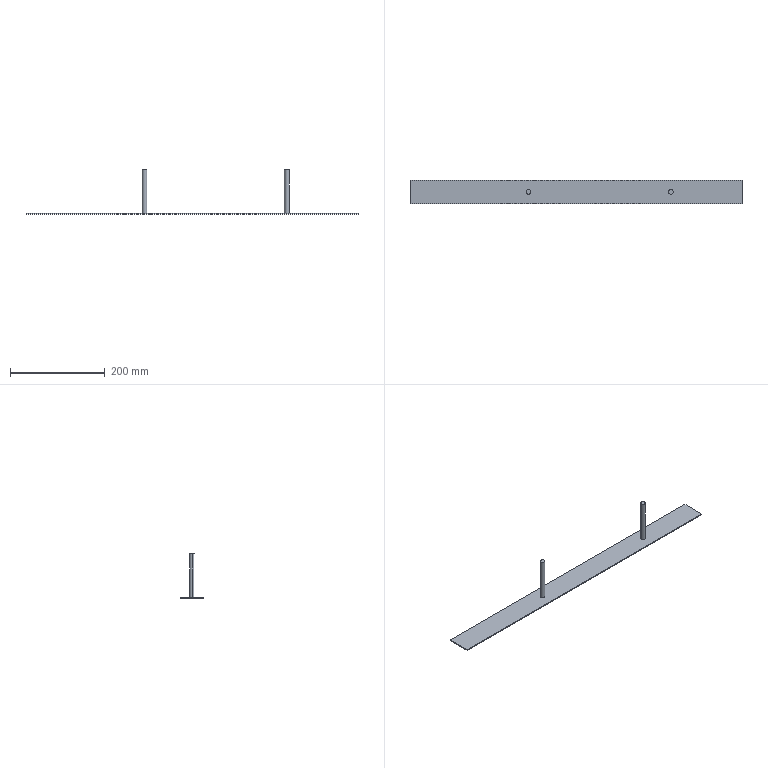Part | STEP file | 1 solid | 12 faces | box 700 x 50 x 93 mm | volume 84294 mm3 | plane 8 | cylinder 4 | commonest cylinder face diameters 10 x4
STEP:
#1=CARTESIAN_POINT('',(0.,0.,0.));
#2=DIRECTION('',(0.,0.,1.));
#3=DIRECTION('',(1.,0.,0.));
#4=AXIS2_PLACEMENT_3D('',#1,#2,#3);
#5=CARTESIAN_POINT('',(195.,0.,2.));
#6=VERTEX_POINT('',#5);
#7=CARTESIAN_POINT('',(205.,0.,2.));
#8=VERTEX_POINT('',#7);
#9=CARTESIAN_POINT('',(200.,0.,2.));
#10=DIRECTION('',(0.,0.,-1.));
#11=DIRECTION('',(1.,0.,0.));
#12=AXIS2_PLACEMENT_3D('',#9,#10,#11);
#13=CIRCLE('',#12,5.);
#14=CARTESIAN_POINT('',(200.,0.,93.));
#15=DIRECTION('',(0.,0.,1.));
#16=DIRECTION('',(1.,0.,0.));
#17=AXIS2_PLACEMENT_3D('',#14,#15,#16);
#18=CYLINDRICAL_SURFACE('',#17,5.);
#19=CARTESIAN_POINT('',(6.283,-91.));
#20=DIRECTION('',(-1.,0.));
#21=VECTOR('',#20,1.);
#22=LINE('',#19,#21);
#23=(GEOMETRIC_REPRESENTATION_CONTEXT(2)PARAMETRIC_REPRESENTATION_CONTEXT()REPRESENTATION_CONTEXT('',''));
#24=DEFINITIONAL_REPRESENTATION('',(#22),#23);
#25=PCURVE('',#18,#24);
#26=CARTESIAN_POINT('',(0.,0.,2.));
#27=DIRECTION('',(0.,0.,1.));
#28=DIRECTION('',(1.,0.,0.));
#29=AXIS2_PLACEMENT_3D('',#26,#27,#28);
#30=PLANE('',#29);
#31=CARTESIAN_POINT('',(205.,0.));
#32=CARTESIAN_POINT('',(205.,-8.66));
#33=CARTESIAN_POINT('',(197.5,-4.33));
#34=CARTESIAN_POINT('',(190.,0.));
#35=CARTESIAN_POINT('',(197.5,4.33));
#36=CARTESIAN_POINT('',(205.,8.66));
#37=CARTESIAN_POINT('',(205.,0.));
#38=(BOUNDED_CURVE()B_SPLINE_CURVE(2,(#31,#32,#33,#34,#35,#36,#37),.UNSPECIFIED.,.T.,.F.)B_SPLINE_CURVE_WITH_KNOTS((1,2,2,2,2,1),(-2.094,0.,2.094,4.189,6.283,8.378),.UNSPECIFIED.)CURVE()GEOMETRIC_REPRESENTATION_ITEM()RATIONAL_B_SPLINE_CURVE((1.,0.5,1.,0.5,1.,0.5,1.))REPRESENTATION_ITEM(''));
#39=(GEOMETRIC_REPRESENTATION_CONTEXT(2)PARAMETRIC_REPRESENTATION_CONTEXT()REPRESENTATION_CONTEXT('',''));
#40=DEFINITIONAL_REPRESENTATION('',(#38),#39);
#41=PCURVE('',#30,#40);
#42=SURFACE_CURVE('',#13,(#25,#41),.PCURVE_S1.);
#43=EDGE_CURVE('',#6,#8,#42,.T.);
#44=ORIENTED_EDGE('',*,*,#43,.F.);
#45=CARTESIAN_POINT('',(195.,0.,93.));
#46=VERTEX_POINT('',#45);
#47=CARTESIAN_POINT('',(195.,0.,93.));
#48=DIRECTION('',(0.,0.,1.));
#49=VECTOR('',#48,1.);
#50=LINE('',#47,#49);
#51=CARTESIAN_POINT('',(3.142,0.));
#52=DIRECTION('',(0.,1.));
#53=VECTOR('',#52,1.);
#54=LINE('',#51,#53);
#55=(GEOMETRIC_REPRESENTATION_CONTEXT(2)PARAMETRIC_REPRESENTATION_CONTEXT()REPRESENTATION_CONTEXT('',''));
#56=DEFINITIONAL_REPRESENTATION('',(#54),#55);
#57=PCURVE('',#18,#56);
#58=CARTESIAN_POINT('',(200.,0.,93.));
#59=DIRECTION('',(0.,0.,1.));
#60=DIRECTION('',(1.,0.,0.));
#61=AXIS2_PLACEMENT_3D('',#58,#59,#60);
#62=CYLINDRICAL_SURFACE('',#61,5.);
#63=CARTESIAN_POINT('',(3.142,0.));
#64=DIRECTION('',(0.,1.));
#65=VECTOR('',#64,1.);
#66=LINE('',#63,#65);
#67=(GEOMETRIC_REPRESENTATION_CONTEXT(2)PARAMETRIC_REPRESENTATION_CONTEXT()REPRESENTATION_CONTEXT('',''));
#68=DEFINITIONAL_REPRESENTATION('',(#66),#67);
#69=PCURVE('',#62,#68);
#70=SURFACE_CURVE('',#50,(#57,#69),.PCURVE_S1.);
#71=EDGE_CURVE('',#6,#46,#70,.T.);
#72=ORIENTED_EDGE('',*,*,#71,.T.);
#73=CARTESIAN_POINT('',(205.,0.,93.));
#74=VERTEX_POINT('',#73);
#75=CARTESIAN_POINT('',(200.,0.,93.));
#76=DIRECTION('',(0.,0.,-1.));
#77=DIRECTION('',(1.,0.,0.));
#78=AXIS2_PLACEMENT_3D('',#75,#76,#77);
#79=CIRCLE('',#78,5.);
#80=CARTESIAN_POINT('',(6.283,0.));
#81=DIRECTION('',(-1.,0.));
#82=VECTOR('',#81,1.);
#83=LINE('',#80,#82);
#84=(GEOMETRIC_REPRESENTATION_CONTEXT(2)PARAMETRIC_REPRESENTATION_CONTEXT()REPRESENTATION_CONTEXT('',''));
#85=DEFINITIONAL_REPRESENTATION('',(#83),#84);
#86=PCURVE('',#18,#85);
#87=CARTESIAN_POINT('',(200.,0.,93.));
#88=DIRECTION('',(0.,0.,1.));
#89=DIRECTION('',(1.,0.,0.));
#90=AXIS2_PLACEMENT_3D('',#87,#88,#89);
#91=PLANE('',#90);
#92=CARTESIAN_POINT('',(5.,0.));
#93=CARTESIAN_POINT('',(5.,-8.66));
#94=CARTESIAN_POINT('',(-2.5,-4.33));
#95=CARTESIAN_POINT('',(-10.,0.));
#96=CARTESIAN_POINT('',(-2.5,4.33));
#97=CARTESIAN_POINT('',(5.,8.66));
#98=CARTESIAN_POINT('',(5.,0.));
#99=(BOUNDED_CURVE()B_SPLINE_CURVE(2,(#92,#93,#94,#95,#96,#97,#98),.UNSPECIFIED.,.T.,.F.)B_SPLINE_CURVE_WITH_KNOTS((1,2,2,2,2,1),(-2.094,0.,2.094,4.189,6.283,8.378),.UNSPECIFIED.)CURVE()GEOMETRIC_REPRESENTATION_ITEM()RATIONAL_B_SPLINE_CURVE((1.,0.5,1.,0.5,1.,0.5,1.))REPRESENTATION_ITEM(''));
#100=(GEOMETRIC_REPRESENTATION_CONTEXT(2)PARAMETRIC_REPRESENTATION_CONTEXT()REPRESENTATION_CONTEXT('',''));
#101=DEFINITIONAL_REPRESENTATION('',(#99),#100);
#102=PCURVE('',#91,#101);
#103=SURFACE_CURVE('',#79,(#86,#102),.PCURVE_S1.);
#104=EDGE_CURVE('',#46,#74,#103,.T.);
#105=ORIENTED_EDGE('',*,*,#104,.T.);
#106=CARTESIAN_POINT('',(205.,0.,93.));
#107=DIRECTION('',(0.,0.,1.));
#108=VECTOR('',#107,1.);
#109=LINE('',#106,#108);
#110=CARTESIAN_POINT('',(0.,0.));
#111=DIRECTION('',(0.,1.));
#112=VECTOR('',#111,1.);
#113=LINE('',#110,#112);
#114=(GEOMETRIC_REPRESENTATION_CONTEXT(2)PARAMETRIC_REPRESENTATION_CONTEXT()REPRESENTATION_CONTEXT('',''));
#115=DEFINITIONAL_REPRESENTATION('',(#113),#114);
#116=PCURVE('',#18,#115);
#117=CARTESIAN_POINT('',(6.283,0.));
#118=DIRECTION('',(0.,1.));
#119=VECTOR('',#118,1.);
#120=LINE('',#117,#119);
#121=(GEOMETRIC_REPRESENTATION_CONTEXT(2)PARAMETRIC_REPRESENTATION_CONTEXT()REPRESENTATION_CONTEXT('',''));
#122=DEFINITIONAL_REPRESENTATION('',(#120),#121);
#123=PCURVE('',#62,#122);
#124=SURFACE_CURVE('',#109,(#116,#123),.PCURVE_S1.);
#125=EDGE_CURVE('',#8,#74,#124,.T.);
#126=ORIENTED_EDGE('',*,*,#125,.F.);
#127=EDGE_LOOP('',(#44,#72,#105,#126));
#128=FACE_BOUND('',#127,.T.);
#129=ADVANCED_FACE('',(#128),#18,.T.);
#130=CARTESIAN_POINT('',(-105.,0.,2.));
#131=VERTEX_POINT('',#130);
#132=CARTESIAN_POINT('',(-95.,0.,2.));
#133=VERTEX_POINT('',#132);
#134=CARTESIAN_POINT('',(-100.,0.,2.));
#135=DIRECTION('',(0.,0.,-1.));
#136=DIRECTION('',(1.,0.,0.));
#137=AXIS2_PLACEMENT_3D('',#134,#135,#136);
#138=CIRCLE('',#137,5.);
#139=CARTESIAN_POINT('',(-100.,0.,93.));
#140=DIRECTION('',(0.,0.,1.));
#141=DIRECTION('',(1.,0.,0.));
#142=AXIS2_PLACEMENT_3D('',#139,#140,#141);
#143=CYLINDRICAL_SURFACE('',#142,5.);
#144=CARTESIAN_POINT('',(6.283,-91.));
#145=DIRECTION('',(-1.,0.));
#146=VECTOR('',#145,1.);
#147=LINE('',#144,#146);
#148=(GEOMETRIC_REPRESENTATION_CONTEXT(2)PARAMETRIC_REPRESENTATION_CONTEXT()REPRESENTATION_CONTEXT('',''));
#149=DEFINITIONAL_REPRESENTATION('',(#147),#148);
#150=PCURVE('',#143,#149);
#151=CARTESIAN_POINT('',(-95.,0.));
#152=CARTESIAN_POINT('',(-95.,-8.66));
#153=CARTESIAN_POINT('',(-102.5,-4.33));
#154=CARTESIAN_POINT('',(-110.,0.));
#155=CARTESIAN_POINT('',(-102.5,4.33));
#156=CARTESIAN_POINT('',(-95.,8.66));
#157=CARTESIAN_POINT('',(-95.,0.));
#158=(BOUNDED_CURVE()B_SPLINE_CURVE(2,(#151,#152,#153,#154,#155,#156,#157),.UNSPECIFIED.,.T.,.F.)B_SPLINE_CURVE_WITH_KNOTS((1,2,2,2,2,1),(-2.094,0.,2.094,4.189,6.283,8.378),.UNSPECIFIED.)CURVE()GEOMETRIC_REPRESENTATION_ITEM()RATIONAL_B_SPLINE_CURVE((1.,0.5,1.,0.5,1.,0.5,1.))REPRESENTATION_ITEM(''));
#159=(GEOMETRIC_REPRESENTATION_CONTEXT(2)PARAMETRIC_REPRESENTATION_CONTEXT()REPRESENTATION_CONTEXT('',''));
#160=DEFINITIONAL_REPRESENTATION('',(#158),#159);
#161=PCURVE('',#30,#160);
#162=SURFACE_CURVE('',#138,(#150,#161),.PCURVE_S1.);
#163=EDGE_CURVE('',#131,#133,#162,.T.);
#164=ORIENTED_EDGE('',*,*,#163,.F.);
#165=CARTESIAN_POINT('',(-105.,0.,93.));
#166=VERTEX_POINT('',#165);
#167=CARTESIAN_POINT('',(-105.,0.,93.));
#168=DIRECTION('',(0.,0.,1.));
#169=VECTOR('',#168,1.);
#170=LINE('',#167,#169);
#171=CARTESIAN_POINT('',(3.142,0.));
#172=DIRECTION('',(0.,1.));
#173=VECTOR('',#172,1.);
#174=LINE('',#171,#173);
#175=(GEOMETRIC_REPRESENTATION_CONTEXT(2)PARAMETRIC_REPRESENTATION_CONTEXT()REPRESENTATION_CONTEXT('',''));
#176=DEFINITIONAL_REPRESENTATION('',(#174),#175);
#177=PCURVE('',#143,#176);
#178=CARTESIAN_POINT('',(-100.,0.,93.));
#179=DIRECTION('',(0.,0.,1.));
#180=DIRECTION('',(1.,0.,0.));
#181=AXIS2_PLACEMENT_3D('',#178,#179,#180);
#182=CYLINDRICAL_SURFACE('',#181,5.);
#183=CARTESIAN_POINT('',(3.142,0.));
#184=DIRECTION('',(0.,1.));
#185=VECTOR('',#184,1.);
#186=LINE('',#183,#185);
#187=(GEOMETRIC_REPRESENTATION_CONTEXT(2)PARAMETRIC_REPRESENTATION_CONTEXT()REPRESENTATION_CONTEXT('',''));
#188=DEFINITIONAL_REPRESENTATION('',(#186),#187);
#189=PCURVE('',#182,#188);
#190=SURFACE_CURVE('',#170,(#177,#189),.PCURVE_S1.);
#191=EDGE_CURVE('',#131,#166,#190,.T.);
#192=ORIENTED_EDGE('',*,*,#191,.T.);
#193=CARTESIAN_POINT('',(-95.,0.,93.));
#194=VERTEX_POINT('',#193);
#195=CARTESIAN_POINT('',(-100.,0.,93.));
#196=DIRECTION('',(0.,0.,-1.));
#197=DIRECTION('',(1.,0.,0.));
#198=AXIS2_PLACEMENT_3D('',#195,#196,#197);
#199=CIRCLE('',#198,5.);
#200=CARTESIAN_POINT('',(6.283,0.));
#201=DIRECTION('',(-1.,0.));
#202=VECTOR('',#201,1.);
#203=LINE('',#200,#202);
#204=(GEOMETRIC_REPRESENTATION_CONTEXT(2)PARAMETRIC_REPRESENTATION_CONTEXT()REPRESENTATION_CONTEXT('',''));
#205=DEFINITIONAL_REPRESENTATION('',(#203),#204);
#206=PCURVE('',#143,#205);
#207=CARTESIAN_POINT('',(-100.,0.,93.));
#208=DIRECTION('',(0.,0.,1.));
#209=DIRECTION('',(1.,0.,0.));
#210=AXIS2_PLACEMENT_3D('',#207,#208,#209);
#211=PLANE('',#210);
#212=CARTESIAN_POINT('',(5.,0.));
#213=CARTESIAN_POINT('',(5.,-8.66));
#214=CARTESIAN_POINT('',(-2.5,-4.33));
#215=CARTESIAN_POINT('',(-10.,0.));
#216=CARTESIAN_POINT('',(-2.5,4.33));
#217=CARTESIAN_POINT('',(5.,8.66));
#218=CARTESIAN_POINT('',(5.,0.));
#219=(BOUNDED_CURVE()B_SPLINE_CURVE(2,(#212,#213,#214,#215,#216,#217,#218),.UNSPECIFIED.,.T.,.F.)B_SPLINE_CURVE_WITH_KNOTS((1,2,2,2,2,1),(-2.094,0.,2.094,4.189,6.283,8.378),.UNSPECIFIED.)CURVE()GEOMETRIC_REPRESENTATION_ITEM()RATIONAL_B_SPLINE_CURVE((1.,0.5,1.,0.5,1.,0.5,1.))REPRESENTATION_ITEM(''));
#220=(GEOMETRIC_REPRESENTATION_CONTEXT(2)PARAMETRIC_REPRESENTATION_CONTEXT()REPRESENTATION_CONTEXT('',''));
#221=DEFINITIONAL_REPRESENTATION('',(#219),#220);
#222=PCURVE('',#211,#221);
#223=SURFACE_CURVE('',#199,(#206,#222),.PCURVE_S1.);
#224=EDGE_CURVE('',#166,#194,#223,.T.);
#225=ORIENTED_EDGE('',*,*,#224,.T.);
#226=CARTESIAN_POINT('',(-95.,0.,93.));
#227=DIRECTION('',(0.,0.,1.));
#228=VECTOR('',#227,1.);
#229=LINE('',#226,#228);
#230=CARTESIAN_POINT('',(0.,0.));
#231=DIRECTION('',(0.,1.));
#232=VECTOR('',#231,1.);
#233=LINE('',#230,#232);
#234=(GEOMETRIC_REPRESENTATION_CONTEXT(2)PARAMETRIC_REPRESENTATION_CONTEXT()REPRESENTATION_CONTEXT('',''));
#235=DEFINITIONAL_REPRESENTATION('',(#233),#234);
#236=PCURVE('',#143,#235);
#237=CARTESIAN_POINT('',(6.283,0.));
#238=DIRECTION('',(0.,1.));
#239=VECTOR('',#238,1.);
#240=LINE('',#237,#239);
#241=(GEOMETRIC_REPRESENTATION_CONTEXT(2)PARAMETRIC_REPRESENTATION_CONTEXT()REPRESENTATION_CONTEXT('',''));
#242=DEFINITIONAL_REPRESENTATION('',(#240),#241);
#243=PCURVE('',#182,#242);
#244=SURFACE_CURVE('',#229,(#236,#243),.PCURVE_S1.);
#245=EDGE_CURVE('',#133,#194,#244,.T.);
#246=ORIENTED_EDGE('',*,*,#245,.F.);
#247=EDGE_LOOP('',(#164,#192,#225,#246));
#248=FACE_BOUND('',#247,.T.);
#249=ADVANCED_FACE('',(#248),#143,.T.);
#250=CARTESIAN_POINT('',(-350.,-25.,0.));
#251=VERTEX_POINT('',#250);
#252=CARTESIAN_POINT('',(350.,-25.,0.));
#253=VERTEX_POINT('',#252);
#254=CARTESIAN_POINT('',(0.,-25.,0.));
#255=DIRECTION('',(1.,0.,0.));
#256=VECTOR('',#255,1.);
#257=LINE('',#254,#256);
#258=CARTESIAN_POINT('',(0.,0.,0.));
#259=DIRECTION('',(0.,0.,1.));
#260=DIRECTION('',(1.,0.,0.));
#261=AXIS2_PLACEMENT_3D('',#258,#259,#260);
#262=PLANE('',#261);
#263=CARTESIAN_POINT('',(0.,-25.));
#264=DIRECTION('',(1.,0.));
#265=VECTOR('',#264,1.);
#266=LINE('',#263,#265);
#267=(GEOMETRIC_REPRESENTATION_CONTEXT(2)PARAMETRIC_REPRESENTATION_CONTEXT()REPRESENTATION_CONTEXT('',''));
#268=DEFINITIONAL_REPRESENTATION('',(#266),#267);
#269=PCURVE('',#262,#268);
#270=CARTESIAN_POINT('',(-350.,-25.,2.));
#271=DIRECTION('',(0.,1.,0.));
#272=DIRECTION('',(0.,0.,1.));
#273=AXIS2_PLACEMENT_3D('',#270,#271,#272);
#274=PLANE('',#273);
#275=CARTESIAN_POINT('',(-2.,350.));
#276=DIRECTION('',(0.,1.));
#277=VECTOR('',#276,1.);
#278=LINE('',#275,#277);
#279=(GEOMETRIC_REPRESENTATION_CONTEXT(2)PARAMETRIC_REPRESENTATION_CONTEXT()REPRESENTATION_CONTEXT('',''));
#280=DEFINITIONAL_REPRESENTATION('',(#278),#279);
#281=PCURVE('',#274,#280);
#282=SURFACE_CURVE('',#257,(#269,#281),.PCURVE_S1.);
#283=EDGE_CURVE('',#251,#253,#282,.T.);
#284=ORIENTED_EDGE('',*,*,#283,.F.);
#285=CARTESIAN_POINT('',(-350.,25.,0.));
#286=VERTEX_POINT('',#285);
#287=CARTESIAN_POINT('',(-350.,0.,0.));
#288=DIRECTION('',(0.,-1.,0.));
#289=VECTOR('',#288,1.);
#290=LINE('',#287,#289);
#291=CARTESIAN_POINT('',(-350.,0.));
#292=DIRECTION('',(0.,-1.));
#293=VECTOR('',#292,1.);
#294=LINE('',#291,#293);
#295=(GEOMETRIC_REPRESENTATION_CONTEXT(2)PARAMETRIC_REPRESENTATION_CONTEXT()REPRESENTATION_CONTEXT('',''));
#296=DEFINITIONAL_REPRESENTATION('',(#294),#295);
#297=PCURVE('',#262,#296);
#298=CARTESIAN_POINT('',(-350.,25.,2.));
#299=DIRECTION('',(1.,0.,0.));
#300=DIRECTION('',(0.,0.,-1.));
#301=AXIS2_PLACEMENT_3D('',#298,#299,#300);
#302=PLANE('',#301);
#303=CARTESIAN_POINT('',(2.,-25.));
#304=DIRECTION('',(0.,-1.));
#305=VECTOR('',#304,1.);
#306=LINE('',#303,#305);
#307=(GEOMETRIC_REPRESENTATION_CONTEXT(2)PARAMETRIC_REPRESENTATION_CONTEXT()REPRESENTATION_CONTEXT('',''));
#308=DEFINITIONAL_REPRESENTATION('',(#306),#307);
#309=PCURVE('',#302,#308);
#310=SURFACE_CURVE('',#290,(#297,#309),.PCURVE_S1.);
#311=EDGE_CURVE('',#286,#251,#310,.T.);
#312=ORIENTED_EDGE('',*,*,#311,.F.);
#313=CARTESIAN_POINT('',(350.,25.,0.));
#314=VERTEX_POINT('',#313);
#315=CARTESIAN_POINT('',(0.,25.,0.));
#316=DIRECTION('',(-1.,0.,0.));
#317=VECTOR('',#316,1.);
#318=LINE('',#315,#317);
#319=CARTESIAN_POINT('',(0.,25.));
#320=DIRECTION('',(-1.,0.));
#321=VECTOR('',#320,1.);
#322=LINE('',#319,#321);
#323=(GEOMETRIC_REPRESENTATION_CONTEXT(2)PARAMETRIC_REPRESENTATION_CONTEXT()REPRESENTATION_CONTEXT('',''));
#324=DEFINITIONAL_REPRESENTATION('',(#322),#323);
#325=PCURVE('',#262,#324);
#326=CARTESIAN_POINT('',(-350.,25.,2.));
#327=DIRECTION('',(0.,-1.,0.));
#328=DIRECTION('',(0.,0.,-1.));
#329=AXIS2_PLACEMENT_3D('',#326,#327,#328);
#330=PLANE('',#329);
#331=CARTESIAN_POINT('',(2.,350.));
#332=DIRECTION('',(0.,-1.));
#333=VECTOR('',#332,1.);
#334=LINE('',#331,#333);
#335=(GEOMETRIC_REPRESENTATION_CONTEXT(2)PARAMETRIC_REPRESENTATION_CONTEXT()REPRESENTATION_CONTEXT('',''));
#336=DEFINITIONAL_REPRESENTATION('',(#334),#335);
#337=PCURVE('',#330,#336);
#338=SURFACE_CURVE('',#318,(#325,#337),.PCURVE_S1.);
#339=EDGE_CURVE('',#314,#286,#338,.T.);
#340=ORIENTED_EDGE('',*,*,#339,.F.);
#341=CARTESIAN_POINT('',(350.,0.,0.));
#342=DIRECTION('',(0.,1.,0.));
#343=VECTOR('',#342,1.);
#344=LINE('',#341,#343);
#345=CARTESIAN_POINT('',(350.,0.));
#346=DIRECTION('',(0.,1.));
#347=VECTOR('',#346,1.);
#348=LINE('',#345,#347);
#349=(GEOMETRIC_REPRESENTATION_CONTEXT(2)PARAMETRIC_REPRESENTATION_CONTEXT()REPRESENTATION_CONTEXT('',''));
#350=DEFINITIONAL_REPRESENTATION('',(#348),#349);
#351=PCURVE('',#262,#350);
#352=CARTESIAN_POINT('',(350.,25.,2.));
#353=DIRECTION('',(-1.,0.,0.));
#354=DIRECTION('',(0.,0.,1.));
#355=AXIS2_PLACEMENT_3D('',#352,#353,#354);
#356=PLANE('',#355);
#357=CARTESIAN_POINT('',(-2.,-25.));
#358=DIRECTION('',(0.,1.));
#359=VECTOR('',#358,1.);
#360=LINE('',#357,#359);
#361=(GEOMETRIC_REPRESENTATION_CONTEXT(2)PARAMETRIC_REPRESENTATION_CONTEXT()REPRESENTATION_CONTEXT('',''));
#362=DEFINITIONAL_REPRESENTATION('',(#360),#361);
#363=PCURVE('',#356,#362);
#364=SURFACE_CURVE('',#344,(#351,#363),.PCURVE_S1.);
#365=EDGE_CURVE('',#253,#314,#364,.T.);
#366=ORIENTED_EDGE('',*,*,#365,.F.);
#367=EDGE_LOOP('',(#284,#312,#340,#366));
#368=FACE_BOUND('',#367,.T.);
#369=ADVANCED_FACE('',(#368),#262,.F.);
#370=CARTESIAN_POINT('',(350.,25.,2.));
#371=VERTEX_POINT('',#370);
#372=CARTESIAN_POINT('',(350.,25.,2.));
#373=DIRECTION('',(0.,0.,-1.));
#374=VECTOR('',#373,1.);
#375=LINE('',#372,#374);
#376=CARTESIAN_POINT('',(0.,0.));
#377=DIRECTION('',(-1.,0.));
#378=VECTOR('',#377,1.);
#379=LINE('',#376,#378);
#380=(GEOMETRIC_REPRESENTATION_CONTEXT(2)PARAMETRIC_REPRESENTATION_CONTEXT()REPRESENTATION_CONTEXT('',''));
#381=DEFINITIONAL_REPRESENTATION('',(#379),#380);
#382=PCURVE('',#356,#381);
#383=CARTESIAN_POINT('',(0.,700.));
#384=DIRECTION('',(1.,0.));
#385=VECTOR('',#384,1.);
#386=LINE('',#383,#385);
#387=(GEOMETRIC_REPRESENTATION_CONTEXT(2)PARAMETRIC_REPRESENTATION_CONTEXT()REPRESENTATION_CONTEXT('',''));
#388=DEFINITIONAL_REPRESENTATION('',(#386),#387);
#389=PCURVE('',#330,#388);
#390=SURFACE_CURVE('',#375,(#382,#389),.PCURVE_S1.);
#391=EDGE_CURVE('',#371,#314,#390,.T.);
#392=ORIENTED_EDGE('',*,*,#391,.F.);
#393=CARTESIAN_POINT('',(350.,-25.,2.));
#394=VERTEX_POINT('',#393);
#395=CARTESIAN_POINT('',(350.,25.,2.));
#396=DIRECTION('',(0.,1.,0.));
#397=VECTOR('',#396,1.);
#398=LINE('',#395,#397);
#399=CARTESIAN_POINT('',(0.,0.));
#400=DIRECTION('',(0.,1.));
#401=VECTOR('',#400,1.);
#402=LINE('',#399,#401);
#403=(GEOMETRIC_REPRESENTATION_CONTEXT(2)PARAMETRIC_REPRESENTATION_CONTEXT()REPRESENTATION_CONTEXT('',''));
#404=DEFINITIONAL_REPRESENTATION('',(#402),#403);
#405=PCURVE('',#356,#404);
#406=CARTESIAN_POINT('',(350.,25.));
#407=DIRECTION('',(0.,1.));
#408=VECTOR('',#407,1.);
#409=LINE('',#406,#408);
#410=(GEOMETRIC_REPRESENTATION_CONTEXT(2)PARAMETRIC_REPRESENTATION_CONTEXT()REPRESENTATION_CONTEXT('',''));
#411=DEFINITIONAL_REPRESENTATION('',(#409),#410);
#412=PCURVE('',#30,#411);
#413=SURFACE_CURVE('',#398,(#405,#412),.PCURVE_S1.);
#414=EDGE_CURVE('',#394,#371,#413,.T.);
#415=ORIENTED_EDGE('',*,*,#414,.F.);
#416=CARTESIAN_POINT('',(350.,-25.,2.));
#417=DIRECTION('',(0.,0.,1.));
#418=VECTOR('',#417,1.);
#419=LINE('',#416,#418);
#420=CARTESIAN_POINT('',(0.,-50.));
#421=DIRECTION('',(1.,0.));
#422=VECTOR('',#421,1.);
#423=LINE('',#420,#422);
#424=(GEOMETRIC_REPRESENTATION_CONTEXT(2)PARAMETRIC_REPRESENTATION_CONTEXT()REPRESENTATION_CONTEXT('',''));
#425=DEFINITIONAL_REPRESENTATION('',(#423),#424);
#426=PCURVE('',#356,#425);
#427=CARTESIAN_POINT('',(0.,700.));
#428=DIRECTION('',(1.,0.));
#429=VECTOR('',#428,1.);
#430=LINE('',#427,#429);
#431=(GEOMETRIC_REPRESENTATION_CONTEXT(2)PARAMETRIC_REPRESENTATION_CONTEXT()REPRESENTATION_CONTEXT('',''));
#432=DEFINITIONAL_REPRESENTATION('',(#430),#431);
#433=PCURVE('',#274,#432);
#434=SURFACE_CURVE('',#419,(#426,#433),.PCURVE_S1.);
#435=EDGE_CURVE('',#253,#394,#434,.T.);
#436=ORIENTED_EDGE('',*,*,#435,.F.);
#437=ORIENTED_EDGE('',*,*,#365,.T.);
#438=EDGE_LOOP('',(#392,#415,#436,#437));
#439=FACE_BOUND('',#438,.T.);
#440=ADVANCED_FACE('',(#439),#356,.F.);
#441=ORIENTED_EDGE('',*,*,#435,.T.);
#442=CARTESIAN_POINT('',(-350.,-25.,2.));
#443=VERTEX_POINT('',#442);
#444=CARTESIAN_POINT('',(-350.,-25.,2.));
#445=DIRECTION('',(1.,0.,0.));
#446=VECTOR('',#445,1.);
#447=LINE('',#444,#446);
#448=CARTESIAN_POINT('',(0.,0.));
#449=DIRECTION('',(0.,1.));
#450=VECTOR('',#449,1.);
#451=LINE('',#448,#450);
#452=(GEOMETRIC_REPRESENTATION_CONTEXT(2)PARAMETRIC_REPRESENTATION_CONTEXT()REPRESENTATION_CONTEXT('',''));
#453=DEFINITIONAL_REPRESENTATION('',(#451),#452);
#454=PCURVE('',#274,#453);
#455=CARTESIAN_POINT('',(-350.,-25.));
#456=DIRECTION('',(1.,0.));
#457=VECTOR('',#456,1.);
#458=LINE('',#455,#457);
#459=(GEOMETRIC_REPRESENTATION_CONTEXT(2)PARAMETRIC_REPRESENTATION_CONTEXT()REPRESENTATION_CONTEXT('',''));
#460=DEFINITIONAL_REPRESENTATION('',(#458),#459);
#461=PCURVE('',#30,#460);
#462=SURFACE_CURVE('',#447,(#454,#461),.PCURVE_S1.);
#463=EDGE_CURVE('',#443,#394,#462,.T.);
#464=ORIENTED_EDGE('',*,*,#463,.F.);
#465=CARTESIAN_POINT('',(-350.,-25.,2.));
#466=DIRECTION('',(0.,0.,1.));
#467=VECTOR('',#466,1.);
#468=LINE('',#465,#467);
#469=CARTESIAN_POINT('',(0.,0.));
#470=DIRECTION('',(1.,0.));
#471=VECTOR('',#470,1.);
#472=LINE('',#469,#471);
#473=(GEOMETRIC_REPRESENTATION_CONTEXT(2)PARAMETRIC_REPRESENTATION_CONTEXT()REPRESENTATION_CONTEXT('',''));
#474=DEFINITIONAL_REPRESENTATION('',(#472),#473);
#475=PCURVE('',#274,#474);
#476=CARTESIAN_POINT('',(0.,-50.));
#477=DIRECTION('',(-1.,0.));
#478=VECTOR('',#477,1.);
#479=LINE('',#476,#478);
#480=(GEOMETRIC_REPRESENTATION_CONTEXT(2)PARAMETRIC_REPRESENTATION_CONTEXT()REPRESENTATION_CONTEXT('',''));
#481=DEFINITIONAL_REPRESENTATION('',(#479),#480);
#482=PCURVE('',#302,#481);
#483=SURFACE_CURVE('',#468,(#475,#482),.PCURVE_S1.);
#484=EDGE_CURVE('',#251,#443,#483,.T.);
#485=ORIENTED_EDGE('',*,*,#484,.F.);
#486=ORIENTED_EDGE('',*,*,#283,.T.);
#487=EDGE_LOOP('',(#441,#464,#485,#486));
#488=FACE_BOUND('',#487,.T.);
#489=ADVANCED_FACE('',(#488),#274,.F.);
#490=ORIENTED_EDGE('',*,*,#484,.T.);
#491=CARTESIAN_POINT('',(-350.,25.,2.));
#492=VERTEX_POINT('',#491);
#493=CARTESIAN_POINT('',(-350.,25.,2.));
#494=DIRECTION('',(0.,-1.,0.));
#495=VECTOR('',#494,1.);
#496=LINE('',#493,#495);
#497=CARTESIAN_POINT('',(0.,0.));
#498=DIRECTION('',(0.,-1.));
#499=VECTOR('',#498,1.);
#500=LINE('',#497,#499);
#501=(GEOMETRIC_REPRESENTATION_CONTEXT(2)PARAMETRIC_REPRESENTATION_CONTEXT()REPRESENTATION_CONTEXT('',''));
#502=DEFINITIONAL_REPRESENTATION('',(#500),#501);
#503=PCURVE('',#302,#502);
#504=CARTESIAN_POINT('',(-350.,25.));
#505=DIRECTION('',(0.,-1.));
#506=VECTOR('',#505,1.);
#507=LINE('',#504,#506);
#508=(GEOMETRIC_REPRESENTATION_CONTEXT(2)PARAMETRIC_REPRESENTATION_CONTEXT()REPRESENTATION_CONTEXT('',''));
#509=DEFINITIONAL_REPRESENTATION('',(#507),#508);
#510=PCURVE('',#30,#509);
#511=SURFACE_CURVE('',#496,(#503,#510),.PCURVE_S1.);
#512=EDGE_CURVE('',#492,#443,#511,.T.);
#513=ORIENTED_EDGE('',*,*,#512,.F.);
#514=CARTESIAN_POINT('',(-350.,25.,2.));
#515=DIRECTION('',(0.,0.,1.));
#516=VECTOR('',#515,1.);
#517=LINE('',#514,#516);
#518=CARTESIAN_POINT('',(0.,0.));
#519=DIRECTION('',(-1.,0.));
#520=VECTOR('',#519,1.);
#521=LINE('',#518,#520);
#522=(GEOMETRIC_REPRESENTATION_CONTEXT(2)PARAMETRIC_REPRESENTATION_CONTEXT()REPRESENTATION_CONTEXT('',''));
#523=DEFINITIONAL_REPRESENTATION('',(#521),#522);
#524=PCURVE('',#302,#523);
#525=CARTESIAN_POINT('',(0.,0.));
#526=DIRECTION('',(-1.,0.));
#527=VECTOR('',#526,1.);
#528=LINE('',#525,#527);
#529=(GEOMETRIC_REPRESENTATION_CONTEXT(2)PARAMETRIC_REPRESENTATION_CONTEXT()REPRESENTATION_CONTEXT('',''));
#530=DEFINITIONAL_REPRESENTATION('',(#528),#529);
#531=PCURVE('',#330,#530);
#532=SURFACE_CURVE('',#517,(#524,#531),.PCURVE_S1.);
#533=EDGE_CURVE('',#286,#492,#532,.T.);
#534=ORIENTED_EDGE('',*,*,#533,.F.);
#535=ORIENTED_EDGE('',*,*,#311,.T.);
#536=EDGE_LOOP('',(#490,#513,#534,#535));
#537=FACE_BOUND('',#536,.T.);
#538=ADVANCED_FACE('',(#537),#302,.F.);
#539=ORIENTED_EDGE('',*,*,#533,.T.);
#540=CARTESIAN_POINT('',(-350.,25.,2.));
#541=DIRECTION('',(-1.,0.,0.));
#542=VECTOR('',#541,1.);
#543=LINE('',#540,#542);
#544=CARTESIAN_POINT('',(0.,0.));
#545=DIRECTION('',(0.,-1.));
#546=VECTOR('',#545,1.);
#547=LINE('',#544,#546);
#548=(GEOMETRIC_REPRESENTATION_CONTEXT(2)PARAMETRIC_REPRESENTATION_CONTEXT()REPRESENTATION_CONTEXT('',''));
#549=DEFINITIONAL_REPRESENTATION('',(#547),#548);
#550=PCURVE('',#330,#549);
#551=CARTESIAN_POINT('',(-350.,25.));
#552=DIRECTION('',(-1.,0.));
#553=VECTOR('',#552,1.);
#554=LINE('',#551,#553);
#555=(GEOMETRIC_REPRESENTATION_CONTEXT(2)PARAMETRIC_REPRESENTATION_CONTEXT()REPRESENTATION_CONTEXT('',''));
#556=DEFINITIONAL_REPRESENTATION('',(#554),#555);
#557=PCURVE('',#30,#556);
#558=SURFACE_CURVE('',#543,(#550,#557),.PCURVE_S1.);
#559=EDGE_CURVE('',#371,#492,#558,.T.);
#560=ORIENTED_EDGE('',*,*,#559,.F.);
#561=ORIENTED_EDGE('',*,*,#391,.T.);
#562=ORIENTED_EDGE('',*,*,#339,.T.);
#563=EDGE_LOOP('',(#539,#560,#561,#562));
#564=FACE_BOUND('',#563,.T.);
#565=ADVANCED_FACE('',(#564),#330,.F.);
#566=CARTESIAN_POINT('',(200.,0.,2.));
#567=DIRECTION('',(0.,0.,-1.));
#568=DIRECTION('',(1.,0.,0.));
#569=AXIS2_PLACEMENT_3D('',#566,#567,#568);
#570=CIRCLE('',#569,5.);
#571=CARTESIAN_POINT('',(205.,0.));
#572=CARTESIAN_POINT('',(205.,-8.66));
#573=CARTESIAN_POINT('',(197.5,-4.33));
#574=CARTESIAN_POINT('',(190.,0.));
#575=CARTESIAN_POINT('',(197.5,4.33));
#576=CARTESIAN_POINT('',(205.,8.66));
#577=CARTESIAN_POINT('',(205.,0.));
#578=(BOUNDED_CURVE()B_SPLINE_CURVE(2,(#571,#572,#573,#574,#575,#576,#577),.UNSPECIFIED.,.T.,.F.)B_SPLINE_CURVE_WITH_KNOTS((1,2,2,2,2,1),(-2.094,0.,2.094,4.189,6.283,8.378),.UNSPECIFIED.)CURVE()GEOMETRIC_REPRESENTATION_ITEM()RATIONAL_B_SPLINE_CURVE((1.,0.5,1.,0.5,1.,0.5,1.))REPRESENTATION_ITEM(''));
#579=(GEOMETRIC_REPRESENTATION_CONTEXT(2)PARAMETRIC_REPRESENTATION_CONTEXT()REPRESENTATION_CONTEXT('',''));
#580=DEFINITIONAL_REPRESENTATION('',(#578),#579);
#581=PCURVE('',#30,#580);
#582=CARTESIAN_POINT('',(6.283,-91.));
#583=DIRECTION('',(-1.,0.));
#584=VECTOR('',#583,1.);
#585=LINE('',#582,#584);
#586=(GEOMETRIC_REPRESENTATION_CONTEXT(2)PARAMETRIC_REPRESENTATION_CONTEXT()REPRESENTATION_CONTEXT('',''));
#587=DEFINITIONAL_REPRESENTATION('',(#585),#586);
#588=PCURVE('',#62,#587);
#589=SURFACE_CURVE('',#570,(#581,#588),.PCURVE_S1.);
#590=EDGE_CURVE('',#8,#6,#589,.T.);
#591=ORIENTED_EDGE('',*,*,#590,.T.);
#592=ORIENTED_EDGE('',*,*,#43,.T.);
#593=EDGE_LOOP('',(#591,#592));
#594=FACE_BOUND('',#593,.T.);
#595=CARTESIAN_POINT('',(-100.,0.,2.));
#596=DIRECTION('',(0.,0.,-1.));
#597=DIRECTION('',(1.,0.,0.));
#598=AXIS2_PLACEMENT_3D('',#595,#596,#597);
#599=CIRCLE('',#598,5.);
#600=CARTESIAN_POINT('',(-95.,0.));
#601=CARTESIAN_POINT('',(-95.,-8.66));
#602=CARTESIAN_POINT('',(-102.5,-4.33));
#603=CARTESIAN_POINT('',(-110.,0.));
#604=CARTESIAN_POINT('',(-102.5,4.33));
#605=CARTESIAN_POINT('',(-95.,8.66));
#606=CARTESIAN_POINT('',(-95.,0.));
#607=(BOUNDED_CURVE()B_SPLINE_CURVE(2,(#600,#601,#602,#603,#604,#605,#606),.UNSPECIFIED.,.T.,.F.)B_SPLINE_CURVE_WITH_KNOTS((1,2,2,2,2,1),(-2.094,0.,2.094,4.189,6.283,8.378),.UNSPECIFIED.)CURVE()GEOMETRIC_REPRESENTATION_ITEM()RATIONAL_B_SPLINE_CURVE((1.,0.5,1.,0.5,1.,0.5,1.))REPRESENTATION_ITEM(''));
#608=(GEOMETRIC_REPRESENTATION_CONTEXT(2)PARAMETRIC_REPRESENTATION_CONTEXT()REPRESENTATION_CONTEXT('',''));
#609=DEFINITIONAL_REPRESENTATION('',(#607),#608);
#610=PCURVE('',#30,#609);
#611=CARTESIAN_POINT('',(6.283,-91.));
#612=DIRECTION('',(-1.,0.));
#613=VECTOR('',#612,1.);
#614=LINE('',#611,#613);
#615=(GEOMETRIC_REPRESENTATION_CONTEXT(2)PARAMETRIC_REPRESENTATION_CONTEXT()REPRESENTATION_CONTEXT('',''));
#616=DEFINITIONAL_REPRESENTATION('',(#614),#615);
#617=PCURVE('',#182,#616);
#618=SURFACE_CURVE('',#599,(#610,#617),.PCURVE_S1.);
#619=EDGE_CURVE('',#133,#131,#618,.T.);
#620=ORIENTED_EDGE('',*,*,#619,.T.);
#621=ORIENTED_EDGE('',*,*,#163,.T.);
#622=EDGE_LOOP('',(#620,#621));
#623=FACE_BOUND('',#622,.T.);
#624=ORIENTED_EDGE('',*,*,#512,.T.);
#625=ORIENTED_EDGE('',*,*,#463,.T.);
#626=ORIENTED_EDGE('',*,*,#414,.T.);
#627=ORIENTED_EDGE('',*,*,#559,.T.);
#628=EDGE_LOOP('',(#624,#625,#626,#627));
#629=FACE_BOUND('',#628,.T.);
#630=ADVANCED_FACE('',(#594,#623,#629),#30,.T.);
#631=ORIENTED_EDGE('',*,*,#71,.F.);
#632=ORIENTED_EDGE('',*,*,#590,.F.);
#633=ORIENTED_EDGE('',*,*,#125,.T.);
#634=CARTESIAN_POINT('',(200.,0.,93.));
#635=DIRECTION('',(0.,0.,-1.));
#636=DIRECTION('',(1.,0.,0.));
#637=AXIS2_PLACEMENT_3D('',#634,#635,#636);
#638=CIRCLE('',#637,5.);
#639=CARTESIAN_POINT('',(6.283,0.));
#640=DIRECTION('',(-1.,0.));
#641=VECTOR('',#640,1.);
#642=LINE('',#639,#641);
#643=(GEOMETRIC_REPRESENTATION_CONTEXT(2)PARAMETRIC_REPRESENTATION_CONTEXT()REPRESENTATION_CONTEXT('',''));
#644=DEFINITIONAL_REPRESENTATION('',(#642),#643);
#645=PCURVE('',#62,#644);
#646=CARTESIAN_POINT('',(5.,0.));
#647=CARTESIAN_POINT('',(5.,-8.66));
#648=CARTESIAN_POINT('',(-2.5,-4.33));
#649=CARTESIAN_POINT('',(-10.,0.));
#650=CARTESIAN_POINT('',(-2.5,4.33));
#651=CARTESIAN_POINT('',(5.,8.66));
#652=CARTESIAN_POINT('',(5.,0.));
#653=(BOUNDED_CURVE()B_SPLINE_CURVE(2,(#646,#647,#648,#649,#650,#651,#652),.UNSPECIFIED.,.T.,.F.)B_SPLINE_CURVE_WITH_KNOTS((1,2,2,2,2,1),(-2.094,0.,2.094,4.189,6.283,8.378),.UNSPECIFIED.)CURVE()GEOMETRIC_REPRESENTATION_ITEM()RATIONAL_B_SPLINE_CURVE((1.,0.5,1.,0.5,1.,0.5,1.))REPRESENTATION_ITEM(''));
#654=(GEOMETRIC_REPRESENTATION_CONTEXT(2)PARAMETRIC_REPRESENTATION_CONTEXT()REPRESENTATION_CONTEXT('',''));
#655=DEFINITIONAL_REPRESENTATION('',(#653),#654);
#656=PCURVE('',#91,#655);
#657=SURFACE_CURVE('',#638,(#645,#656),.PCURVE_S1.);
#658=EDGE_CURVE('',#74,#46,#657,.T.);
#659=ORIENTED_EDGE('',*,*,#658,.T.);
#660=EDGE_LOOP('',(#631,#632,#633,#659));
#661=FACE_BOUND('',#660,.T.);
#662=ADVANCED_FACE('',(#661),#62,.T.);
#663=ORIENTED_EDGE('',*,*,#191,.F.);
#664=ORIENTED_EDGE('',*,*,#619,.F.);
#665=ORIENTED_EDGE('',*,*,#245,.T.);
#666=CARTESIAN_POINT('',(-100.,0.,93.));
#667=DIRECTION('',(0.,0.,-1.));
#668=DIRECTION('',(1.,0.,0.));
#669=AXIS2_PLACEMENT_3D('',#666,#667,#668);
#670=CIRCLE('',#669,5.);
#671=CARTESIAN_POINT('',(6.283,0.));
#672=DIRECTION('',(-1.,0.));
#673=VECTOR('',#672,1.);
#674=LINE('',#671,#673);
#675=(GEOMETRIC_REPRESENTATION_CONTEXT(2)PARAMETRIC_REPRESENTATION_CONTEXT()REPRESENTATION_CONTEXT('',''));
#676=DEFINITIONAL_REPRESENTATION('',(#674),#675);
#677=PCURVE('',#182,#676);
#678=CARTESIAN_POINT('',(5.,0.));
#679=CARTESIAN_POINT('',(5.,-8.66));
#680=CARTESIAN_POINT('',(-2.5,-4.33));
#681=CARTESIAN_POINT('',(-10.,0.));
#682=CARTESIAN_POINT('',(-2.5,4.33));
#683=CARTESIAN_POINT('',(5.,8.66));
#684=CARTESIAN_POINT('',(5.,0.));
#685=(BOUNDED_CURVE()B_SPLINE_CURVE(2,(#678,#679,#680,#681,#682,#683,#684),.UNSPECIFIED.,.T.,.F.)B_SPLINE_CURVE_WITH_KNOTS((1,2,2,2,2,1),(-2.094,0.,2.094,4.189,6.283,8.378),.UNSPECIFIED.)CURVE()GEOMETRIC_REPRESENTATION_ITEM()RATIONAL_B_SPLINE_CURVE((1.,0.5,1.,0.5,1.,0.5,1.))REPRESENTATION_ITEM(''));
#686=(GEOMETRIC_REPRESENTATION_CONTEXT(2)PARAMETRIC_REPRESENTATION_CONTEXT()REPRESENTATION_CONTEXT('',''));
#687=DEFINITIONAL_REPRESENTATION('',(#685),#686);
#688=PCURVE('',#211,#687);
#689=SURFACE_CURVE('',#670,(#677,#688),.PCURVE_S1.);
#690=EDGE_CURVE('',#194,#166,#689,.T.);
#691=ORIENTED_EDGE('',*,*,#690,.T.);
#692=EDGE_LOOP('',(#663,#664,#665,#691));
#693=FACE_BOUND('',#692,.T.);
#694=ADVANCED_FACE('',(#693),#182,.T.);
#695=ORIENTED_EDGE('',*,*,#658,.F.);
#696=ORIENTED_EDGE('',*,*,#104,.F.);
#697=EDGE_LOOP('',(#695,#696));
#698=FACE_BOUND('',#697,.T.);
#699=ADVANCED_FACE('',(#698),#91,.T.);
#700=ORIENTED_EDGE('',*,*,#690,.F.);
#701=ORIENTED_EDGE('',*,*,#224,.F.);
#702=EDGE_LOOP('',(#700,#701));
#703=FACE_BOUND('',#702,.T.);
#704=ADVANCED_FACE('',(#703),#211,.T.);
#705=CLOSED_SHELL('',(#129,#249,#369,#440,#489,#538,#565,#630,#662,#694,#699,#704));
#706=MANIFOLD_SOLID_BREP('',#705);
#707=(LENGTH_UNIT()NAMED_UNIT(*)SI_UNIT(.MILLI.,.METRE.));
#708=UNCERTAINTY_MEASURE_WITH_UNIT(LENGTH_MEASURE(0.0000001),#707,'','');
#709=(NAMED_UNIT(*)PLANE_ANGLE_UNIT()SI_UNIT($,.RADIAN.));
#710=(NAMED_UNIT(*)SI_UNIT($,.STERADIAN.)SOLID_ANGLE_UNIT());
#711=(GEOMETRIC_REPRESENTATION_CONTEXT(3)GLOBAL_UNCERTAINTY_ASSIGNED_CONTEXT((#708))GLOBAL_UNIT_ASSIGNED_CONTEXT((#707,#709,#710))REPRESENTATION_CONTEXT('',''));
#712=ADVANCED_BREP_SHAPE_REPRESENTATION('',(#4,#706),#711);